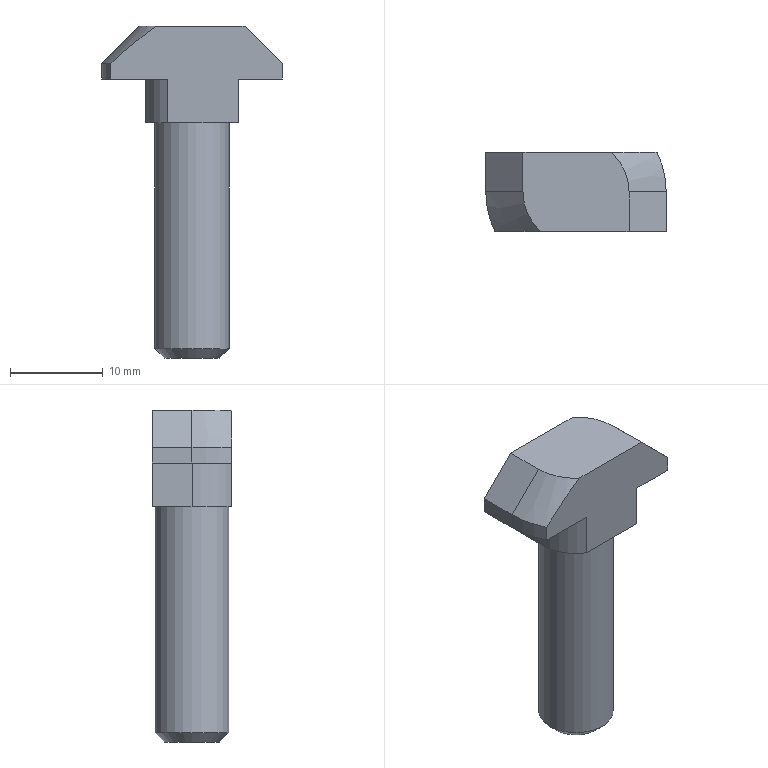Part | STEP file | 1_23 | 1 solid | 21 faces | box 19.4 x 8.5 x 35.7 mm | volume 2417 mm3 | plane 13 | cylinder 5 | cone 3 | commonest cylinder face diameters 10 x2 19.4 x2 8 x1